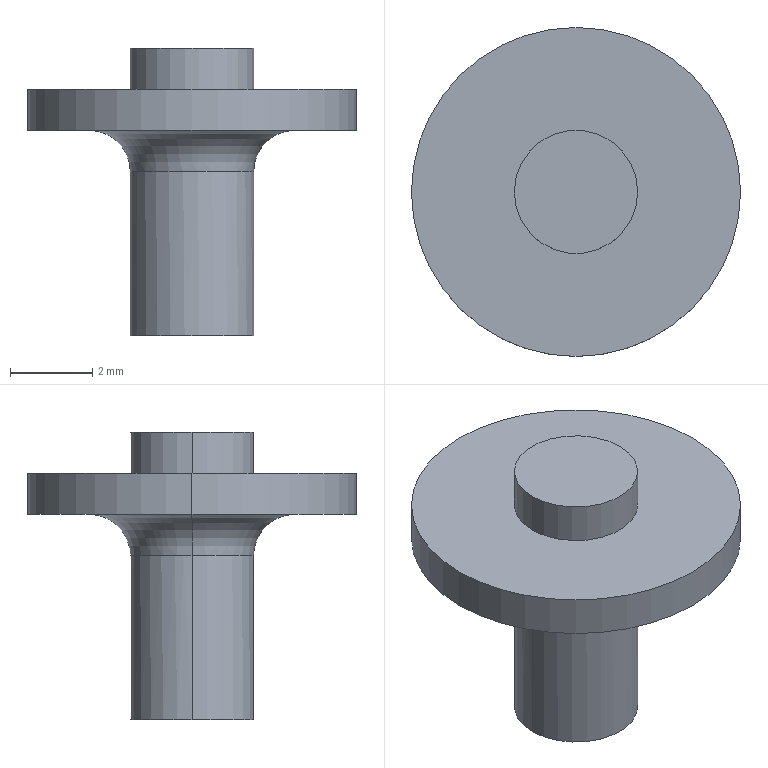Part | SolidWorks | features ICE 3, Extrusion 1, RevCut 1 | 1 solid | 13 faces | box 8 x 8 x 7 mm | volume 95.001 mm3 | cylinder 6 | plane 4 | torus 3 | commonest cylinder face diameters 3 x4 8 x2
STEP:
#1=CARTESIAN_POINT('',(-1.5,0.,-6.));
#2=VERTEX_POINT('',#1);
#3=CARTESIAN_POINT('',(1.5,0.,-6.));
#4=VERTEX_POINT('',#3);
#5=CARTESIAN_POINT('',(0.,0.,-6.));
#6=DIRECTION('',(0.,0.,-1.));
#7=DIRECTION('',(-1.,0.,0.));
#8=AXIS2_PLACEMENT_3D('',#5,#6,#7);
#9=CIRCLE('',#8,1.5);
#10=EDGE_CURVE('',#2,#4,#9,.T.);
#11=ORIENTED_EDGE('',*,*,#10,.F.);
#12=CARTESIAN_POINT('',(-1.5,0.,-2.003));
#13=VERTEX_POINT('',#12);
#14=CARTESIAN_POINT('',(-1.5,0.,-6.));
#15=DIRECTION('',(0.,0.,1.));
#16=VECTOR('',#15,1000.);
#17=LINE('',#14,#16);
#18=EDGE_CURVE('',#2,#13,#17,.T.);
#19=ORIENTED_EDGE('',*,*,#18,.T.);
#20=CARTESIAN_POINT('',(1.5,0.,-2.003));
#21=VERTEX_POINT('',#20);
#22=CARTESIAN_POINT('',(1.5,0.,-2.003));
#23=CARTESIAN_POINT('',(1.5,0.1963,-2.003));
#24=CARTESIAN_POINT('',(1.461,0.3926,-2.003));
#25=CARTESIAN_POINT('',(1.311,0.7554,-2.003));
#26=CARTESIAN_POINT('',(1.2,0.9218,-2.003));
#27=CARTESIAN_POINT('',(0.9218,1.2,-2.003));
#28=CARTESIAN_POINT('',(0.7554,1.311,-2.003));
#29=CARTESIAN_POINT('',(0.3926,1.461,-2.003));
#30=CARTESIAN_POINT('',(0.1963,1.5,-2.003));
#31=CARTESIAN_POINT('',(-0.1963,1.5,-2.003));
#32=CARTESIAN_POINT('',(-0.3926,1.461,-2.003));
#33=CARTESIAN_POINT('',(-0.7554,1.311,-2.003));
#34=CARTESIAN_POINT('',(-0.9218,1.2,-2.003));
#35=CARTESIAN_POINT('',(-1.2,0.9218,-2.003));
#36=CARTESIAN_POINT('',(-1.311,0.7554,-2.003));
#37=CARTESIAN_POINT('',(-1.461,0.3926,-2.003));
#38=CARTESIAN_POINT('',(-1.5,0.1963,-2.003));
#39=CARTESIAN_POINT('',(-1.5,0.,-2.003));
#40=B_SPLINE_CURVE_WITH_KNOTS('',3,(#22,#23,#24,#25,#26,#27,#28,#29,#30,#31,#32,#33,#34,#35,#36,#37,#38,#39),.UNSPECIFIED.,.F.,.F.,(4,2,2,2,2,2,2,2,4),(0.,0.0625,0.125,0.1875,0.25,0.3125,0.375,0.4375,0.5),.UNSPECIFIED.);
#41=EDGE_CURVE('',#21,#13,#40,.T.);
#42=ORIENTED_EDGE('',*,*,#41,.F.);
#43=CARTESIAN_POINT('',(1.5,0.,-6.));
#44=DIRECTION('',(0.,0.,1.));
#45=VECTOR('',#44,1000.);
#46=LINE('',#43,#45);
#47=EDGE_CURVE('',#4,#21,#46,.T.);
#48=ORIENTED_EDGE('',*,*,#47,.F.);
#49=EDGE_LOOP('',(#11,#19,#42,#48));
#50=FACE_OUTER_BOUND('',#49,.T.);
#51=CARTESIAN_POINT('',(0.,0.,-6.));
#52=DIRECTION('',(0.,0.,1.));
#53=DIRECTION('',(1.,0.,0.));
#54=AXIS2_PLACEMENT_3D('',#51,#52,#53);
#55=CYLINDRICAL_SURFACE('',#54,1.5);
#56=ADVANCED_FACE('',(#50),#55,.T.);
#57=CARTESIAN_POINT('',(-2.5,0.,-1.));
#58=VERTEX_POINT('',#57);
#59=CARTESIAN_POINT('',(2.5,0.,-1.));
#60=VERTEX_POINT('',#59);
#61=CARTESIAN_POINT('',(0.,0.,-1.));
#62=DIRECTION('',(0.,0.,1.));
#63=DIRECTION('',(1.,0.,0.));
#64=AXIS2_PLACEMENT_3D('',#61,#62,#63);
#65=CIRCLE('',#64,2.5);
#66=EDGE_CURVE('',#58,#60,#65,.T.);
#67=ORIENTED_EDGE('',*,*,#66,.F.);
#68=CARTESIAN_POINT('',(-2.5,0.,-2.));
#69=DIRECTION('',(0.,1.,0.));
#70=DIRECTION('',(-1.,0.,0.));
#71=AXIS2_PLACEMENT_3D('',#68,#69,#70);
#72=CIRCLE('',#71,1.);
#73=EDGE_CURVE('',#58,#13,#72,.T.);
#74=ORIENTED_EDGE('',*,*,#73,.T.);
#75=CARTESIAN_POINT('',(-1.5,0.,-2.003));
#76=CARTESIAN_POINT('',(-1.5,-0.1963,-2.));
#77=CARTESIAN_POINT('',(-1.461,-0.3926,-2.));
#78=CARTESIAN_POINT('',(-1.311,-0.7554,-2.));
#79=CARTESIAN_POINT('',(-1.199,-0.9218,-2.));
#80=CARTESIAN_POINT('',(-0.9218,-1.199,-2.));
#81=CARTESIAN_POINT('',(-0.7554,-1.311,-2.));
#82=CARTESIAN_POINT('',(-0.3926,-1.461,-2.));
#83=CARTESIAN_POINT('',(-0.1963,-1.5,-2.));
#84=CARTESIAN_POINT('',(0.1963,-1.5,-2.));
#85=CARTESIAN_POINT('',(0.3926,-1.461,-2.));
#86=CARTESIAN_POINT('',(0.7554,-1.311,-2.));
#87=CARTESIAN_POINT('',(0.9218,-1.199,-2.));
#88=CARTESIAN_POINT('',(1.199,-0.9218,-2.));
#89=CARTESIAN_POINT('',(1.311,-0.7554,-2.));
#90=CARTESIAN_POINT('',(1.461,-0.3926,-2.));
#91=CARTESIAN_POINT('',(1.5,-0.1963,-2.));
#92=CARTESIAN_POINT('',(1.5,0.,-2.003));
#93=B_SPLINE_CURVE_WITH_KNOTS('',3,(#75,#76,#77,#78,#79,#80,#81,#82,#83,#84,#85,#86,#87,#88,#89,#90,#91,#92),.UNSPECIFIED.,.F.,.F.,(4,2,2,2,2,2,2,2,4),(0.,0.125,0.25,0.375,0.5,0.625,0.75,0.875,1.),.UNSPECIFIED.);
#94=EDGE_CURVE('',#13,#21,#93,.T.);
#95=ORIENTED_EDGE('',*,*,#94,.T.);
#96=CARTESIAN_POINT('',(2.5,0.,-2.));
#97=DIRECTION('',(0.,-1.,0.));
#98=DIRECTION('',(0.,0.,-1.));
#99=AXIS2_PLACEMENT_3D('',#96,#97,#98);
#100=CIRCLE('',#99,1.);
#101=EDGE_CURVE('',#60,#21,#100,.T.);
#102=ORIENTED_EDGE('',*,*,#101,.F.);
#103=EDGE_LOOP('',(#67,#74,#95,#102));
#104=FACE_OUTER_BOUND('',#103,.T.);
#105=CARTESIAN_POINT('',(0.,0.,-2.));
#106=DIRECTION('',(0.,0.,1.));
#107=DIRECTION('',(1.,0.,0.));
#108=AXIS2_PLACEMENT_3D('',#105,#106,#107);
#109=TOROIDAL_SURFACE('',#108,2.5,1.);
#110=ADVANCED_FACE('',(#104),#109,.F.);
#111=CARTESIAN_POINT('',(-4.,0.,-1.));
#112=VERTEX_POINT('',#111);
#113=CARTESIAN_POINT('',(4.,0.,-1.));
#114=VERTEX_POINT('',#113);
#115=CARTESIAN_POINT('',(0.,0.,-1.));
#116=DIRECTION('',(0.,0.,-1.));
#117=DIRECTION('',(-1.,0.,0.));
#118=AXIS2_PLACEMENT_3D('',#115,#116,#117);
#119=CIRCLE('',#118,4.);
#120=EDGE_CURVE('',#112,#114,#119,.T.);
#121=ORIENTED_EDGE('',*,*,#120,.F.);
#122=CARTESIAN_POINT('',(-4.,0.,0.));
#123=VERTEX_POINT('',#122);
#124=CARTESIAN_POINT('',(-4.,0.,-1.));
#125=DIRECTION('',(0.,0.,1.));
#126=VECTOR('',#125,1000.);
#127=LINE('',#124,#126);
#128=EDGE_CURVE('',#112,#123,#127,.T.);
#129=ORIENTED_EDGE('',*,*,#128,.T.);
#130=CARTESIAN_POINT('',(4.,0.,0.));
#131=VERTEX_POINT('',#130);
#132=CARTESIAN_POINT('',(0.,0.,0.));
#133=DIRECTION('',(0.,0.,-1.));
#134=DIRECTION('',(-1.,0.,0.));
#135=AXIS2_PLACEMENT_3D('',#132,#133,#134);
#136=CIRCLE('',#135,4.);
#137=EDGE_CURVE('',#123,#131,#136,.T.);
#138=ORIENTED_EDGE('',*,*,#137,.T.);
#139=CARTESIAN_POINT('',(4.,0.,-1.));
#140=DIRECTION('',(0.,0.,1.));
#141=VECTOR('',#140,1000.);
#142=LINE('',#139,#141);
#143=EDGE_CURVE('',#114,#131,#142,.T.);
#144=ORIENTED_EDGE('',*,*,#143,.F.);
#145=EDGE_LOOP('',(#121,#129,#138,#144));
#146=FACE_OUTER_BOUND('',#145,.T.);
#147=CARTESIAN_POINT('',(0.,0.,-1.));
#148=DIRECTION('',(0.,0.,1.));
#149=DIRECTION('',(1.,0.,0.));
#150=AXIS2_PLACEMENT_3D('',#147,#148,#149);
#151=CYLINDRICAL_SURFACE('',#150,4.);
#152=ADVANCED_FACE('',(#146),#151,.T.);
#153=CARTESIAN_POINT('',(1.5,0.,1.));
#154=VERTEX_POINT('',#153);
#155=CARTESIAN_POINT('',(-1.5,0.,1.));
#156=VERTEX_POINT('',#155);
#157=CARTESIAN_POINT('',(0.,0.,1.));
#158=DIRECTION('',(0.,0.,1.));
#159=DIRECTION('',(1.,0.,0.));
#160=AXIS2_PLACEMENT_3D('',#157,#158,#159);
#161=CIRCLE('',#160,1.5);
#162=EDGE_CURVE('',#154,#156,#161,.T.);
#163=ORIENTED_EDGE('',*,*,#162,.F.);
#164=CARTESIAN_POINT('',(1.5,0.,0.));
#165=VERTEX_POINT('',#164);
#166=CARTESIAN_POINT('',(1.5,0.,1.));
#167=DIRECTION('',(0.,0.,-1.));
#168=VECTOR('',#167,1000.);
#169=LINE('',#166,#168);
#170=EDGE_CURVE('',#154,#165,#169,.T.);
#171=ORIENTED_EDGE('',*,*,#170,.T.);
#172=CARTESIAN_POINT('',(-1.5,0.,0.));
#173=VERTEX_POINT('',#172);
#174=CARTESIAN_POINT('',(0.,0.,0.));
#175=DIRECTION('',(0.,0.,1.));
#176=DIRECTION('',(1.,0.,0.));
#177=AXIS2_PLACEMENT_3D('',#174,#175,#176);
#178=CIRCLE('',#177,1.5);
#179=EDGE_CURVE('',#165,#173,#178,.T.);
#180=ORIENTED_EDGE('',*,*,#179,.T.);
#181=CARTESIAN_POINT('',(-1.5,0.,1.));
#182=DIRECTION('',(0.,0.,-1.));
#183=VECTOR('',#182,1000.);
#184=LINE('',#181,#183);
#185=EDGE_CURVE('',#156,#173,#184,.T.);
#186=ORIENTED_EDGE('',*,*,#185,.F.);
#187=EDGE_LOOP('',(#163,#171,#180,#186));
#188=FACE_OUTER_BOUND('',#187,.T.);
#189=CARTESIAN_POINT('',(0.,0.,1.));
#190=DIRECTION('',(0.,0.,-1.));
#191=DIRECTION('',(-1.,0.,0.));
#192=AXIS2_PLACEMENT_3D('',#189,#190,#191);
#193=CYLINDRICAL_SURFACE('',#192,1.5);
#194=ADVANCED_FACE('',(#188),#193,.T.);
#195=ORIENTED_EDGE('',*,*,#170,.F.);
#196=CARTESIAN_POINT('',(0.,0.,1.));
#197=DIRECTION('',(0.,0.,1.));
#198=DIRECTION('',(1.,0.,0.));
#199=AXIS2_PLACEMENT_3D('',#196,#197,#198);
#200=CIRCLE('',#199,1.5);
#201=EDGE_CURVE('',#156,#154,#200,.T.);
#202=ORIENTED_EDGE('',*,*,#201,.F.);
#203=ORIENTED_EDGE('',*,*,#185,.T.);
#204=CARTESIAN_POINT('',(0.,0.,0.));
#205=DIRECTION('',(0.,0.,1.));
#206=DIRECTION('',(1.,0.,0.));
#207=AXIS2_PLACEMENT_3D('',#204,#205,#206);
#208=CIRCLE('',#207,1.5);
#209=EDGE_CURVE('',#173,#165,#208,.T.);
#210=ORIENTED_EDGE('',*,*,#209,.T.);
#211=EDGE_LOOP('',(#195,#202,#203,#210));
#212=FACE_OUTER_BOUND('',#211,.T.);
#213=CARTESIAN_POINT('',(0.,0.,1.));
#214=DIRECTION('',(0.,0.,-1.));
#215=DIRECTION('',(-1.,0.,0.));
#216=AXIS2_PLACEMENT_3D('',#213,#214,#215);
#217=CYLINDRICAL_SURFACE('',#216,1.5);
#218=ADVANCED_FACE('',(#212),#217,.T.);
#219=ORIENTED_EDGE('',*,*,#201,.T.);
#220=ORIENTED_EDGE('',*,*,#162,.T.);
#221=EDGE_LOOP('',(#219,#220));
#222=FACE_OUTER_BOUND('',#221,.T.);
#223=CARTESIAN_POINT('',(0.,0.,1.));
#224=DIRECTION('',(0.,0.,1.));
#225=DIRECTION('',(1.,0.,0.));
#226=AXIS2_PLACEMENT_3D('',#223,#224,#225);
#227=PLANE('',#226);
#228=ADVANCED_FACE('',(#222),#227,.T.);
#229=ORIENTED_EDGE('',*,*,#128,.F.);
#230=CARTESIAN_POINT('',(0.,0.,-1.));
#231=DIRECTION('',(0.,0.,-1.));
#232=DIRECTION('',(-1.,0.,0.));
#233=AXIS2_PLACEMENT_3D('',#230,#231,#232);
#234=CIRCLE('',#233,4.);
#235=EDGE_CURVE('',#114,#112,#234,.T.);
#236=ORIENTED_EDGE('',*,*,#235,.F.);
#237=ORIENTED_EDGE('',*,*,#143,.T.);
#238=CARTESIAN_POINT('',(0.,0.,0.));
#239=DIRECTION('',(0.,0.,-1.));
#240=DIRECTION('',(-1.,0.,0.));
#241=AXIS2_PLACEMENT_3D('',#238,#239,#240);
#242=CIRCLE('',#241,4.);
#243=EDGE_CURVE('',#131,#123,#242,.T.);
#244=ORIENTED_EDGE('',*,*,#243,.T.);
#245=EDGE_LOOP('',(#229,#236,#237,#244));
#246=FACE_OUTER_BOUND('',#245,.T.);
#247=CARTESIAN_POINT('',(0.,0.,-1.));
#248=DIRECTION('',(0.,0.,1.));
#249=DIRECTION('',(1.,0.,0.));
#250=AXIS2_PLACEMENT_3D('',#247,#248,#249);
#251=CYLINDRICAL_SURFACE('',#250,4.);
#252=ADVANCED_FACE('',(#246),#251,.T.);
#253=CARTESIAN_POINT('',(0.,0.,-1.));
#254=DIRECTION('',(0.,0.,1.));
#255=DIRECTION('',(1.,0.,0.));
#256=AXIS2_PLACEMENT_3D('',#253,#254,#255);
#257=CIRCLE('',#256,2.5);
#258=EDGE_CURVE('',#60,#58,#257,.T.);
#259=ORIENTED_EDGE('',*,*,#258,.T.);
#260=ORIENTED_EDGE('',*,*,#66,.T.);
#261=EDGE_LOOP('',(#259,#260));
#262=FACE_BOUND('',#261,.T.);
#263=ORIENTED_EDGE('',*,*,#235,.T.);
#264=ORIENTED_EDGE('',*,*,#120,.T.);
#265=EDGE_LOOP('',(#263,#264));
#266=FACE_OUTER_BOUND('',#265,.T.);
#267=CARTESIAN_POINT('',(0.,0.,-1.));
#268=DIRECTION('',(0.,0.,-1.));
#269=DIRECTION('',(-1.,0.,0.));
#270=AXIS2_PLACEMENT_3D('',#267,#268,#269);
#271=PLANE('',#270);
#272=ADVANCED_FACE('',(#262,#266),#271,.T.);
#273=ORIENTED_EDGE('',*,*,#209,.F.);
#274=ORIENTED_EDGE('',*,*,#179,.F.);
#275=EDGE_LOOP('',(#273,#274));
#276=FACE_BOUND('',#275,.T.);
#277=ORIENTED_EDGE('',*,*,#243,.F.);
#278=ORIENTED_EDGE('',*,*,#137,.F.);
#279=EDGE_LOOP('',(#277,#278));
#280=FACE_OUTER_BOUND('',#279,.T.);
#281=CARTESIAN_POINT('',(0.,0.,0.));
#282=DIRECTION('',(0.,0.,-1.));
#283=DIRECTION('',(-1.,0.,0.));
#284=AXIS2_PLACEMENT_3D('',#281,#282,#283);
#285=PLANE('',#284);
#286=ADVANCED_FACE('',(#276,#280),#285,.F.);
#287=ORIENTED_EDGE('',*,*,#41,.T.);
#288=CARTESIAN_POINT('',(0.,0.,-2.));
#289=DIRECTION('',(0.,0.,1.));
#290=DIRECTION('',(1.,0.,0.));
#291=AXIS2_PLACEMENT_3D('',#288,#289,#290);
#292=CIRCLE('',#291,1.5);
#293=EDGE_CURVE('',#21,#13,#292,.T.);
#294=ORIENTED_EDGE('',*,*,#293,.F.);
#295=EDGE_LOOP('',(#287,#294));
#296=FACE_OUTER_BOUND('',#295,.T.);
#297=CARTESIAN_POINT('',(0.,0.,-2.));
#298=DIRECTION('',(0.,0.,1.));
#299=DIRECTION('',(1.,0.,0.));
#300=AXIS2_PLACEMENT_3D('',#297,#298,#299);
#301=TOROIDAL_SURFACE('',#300,2.5,1.);
#302=ADVANCED_FACE('',(#296),#301,.F.);
#303=ORIENTED_EDGE('',*,*,#73,.F.);
#304=ORIENTED_EDGE('',*,*,#258,.F.);
#305=ORIENTED_EDGE('',*,*,#101,.T.);
#306=ORIENTED_EDGE('',*,*,#293,.T.);
#307=EDGE_LOOP('',(#303,#304,#305,#306));
#308=FACE_OUTER_BOUND('',#307,.T.);
#309=CARTESIAN_POINT('',(0.,0.,-2.));
#310=DIRECTION('',(0.,0.,1.));
#311=DIRECTION('',(1.,0.,0.));
#312=AXIS2_PLACEMENT_3D('',#309,#310,#311);
#313=TOROIDAL_SURFACE('',#312,2.5,1.);
#314=ADVANCED_FACE('',(#308),#313,.F.);
#315=CARTESIAN_POINT('',(0.,0.,-6.));
#316=DIRECTION('',(0.,0.,-1.));
#317=DIRECTION('',(-1.,0.,0.));
#318=AXIS2_PLACEMENT_3D('',#315,#316,#317);
#319=CIRCLE('',#318,1.5);
#320=EDGE_CURVE('',#4,#2,#319,.T.);
#321=ORIENTED_EDGE('',*,*,#320,.T.);
#322=ORIENTED_EDGE('',*,*,#10,.T.);
#323=EDGE_LOOP('',(#321,#322));
#324=FACE_OUTER_BOUND('',#323,.T.);
#325=CARTESIAN_POINT('',(0.,0.,-6.));
#326=DIRECTION('',(0.,0.,-1.));
#327=DIRECTION('',(-1.,0.,0.));
#328=AXIS2_PLACEMENT_3D('',#325,#326,#327);
#329=PLANE('',#328);
#330=ADVANCED_FACE('',(#324),#329,.T.);
#331=ORIENTED_EDGE('',*,*,#18,.F.);
#332=ORIENTED_EDGE('',*,*,#320,.F.);
#333=ORIENTED_EDGE('',*,*,#47,.T.);
#334=ORIENTED_EDGE('',*,*,#94,.F.);
#335=EDGE_LOOP('',(#331,#332,#333,#334));
#336=FACE_OUTER_BOUND('',#335,.T.);
#337=CARTESIAN_POINT('',(0.,0.,-6.));
#338=DIRECTION('',(0.,0.,1.));
#339=DIRECTION('',(1.,0.,0.));
#340=AXIS2_PLACEMENT_3D('',#337,#338,#339);
#341=CYLINDRICAL_SURFACE('',#340,1.5);
#342=ADVANCED_FACE('',(#336),#341,.T.);
#343=CLOSED_SHELL('',(#56,#110,#152,#194,#218,#228,#252,#272,#286,#302,#314,#330,#342));
#344=MANIFOLD_SOLID_BREP('',#343);
#345=CARTESIAN_POINT('',(0.,0.,0.));
#346=DIRECTION('',(0.,0.,1.));
#347=DIRECTION('',(1.,0.,0.));
#348=AXIS2_PLACEMENT_3D('',#345,#346,#347);
#349=(LENGTH_UNIT()NAMED_UNIT(*)SI_UNIT(.MILLI.,.METRE.));
#350=UNCERTAINTY_MEASURE_WITH_UNIT(LENGTH_MEASURE(0.00001),#349,'','');
#351=(NAMED_UNIT(*)PLANE_ANGLE_UNIT()SI_UNIT($,.RADIAN.));
#352=(NAMED_UNIT(*)SI_UNIT($,.STERADIAN.)SOLID_ANGLE_UNIT());
#353=(GEOMETRIC_REPRESENTATION_CONTEXT(3)GLOBAL_UNCERTAINTY_ASSIGNED_CONTEXT((#350))GLOBAL_UNIT_ASSIGNED_CONTEXT((#349,#351,#352))REPRESENTATION_CONTEXT('',''));
#354=ADVANCED_BREP_SHAPE_REPRESENTATION('',(#344,#348),#353);